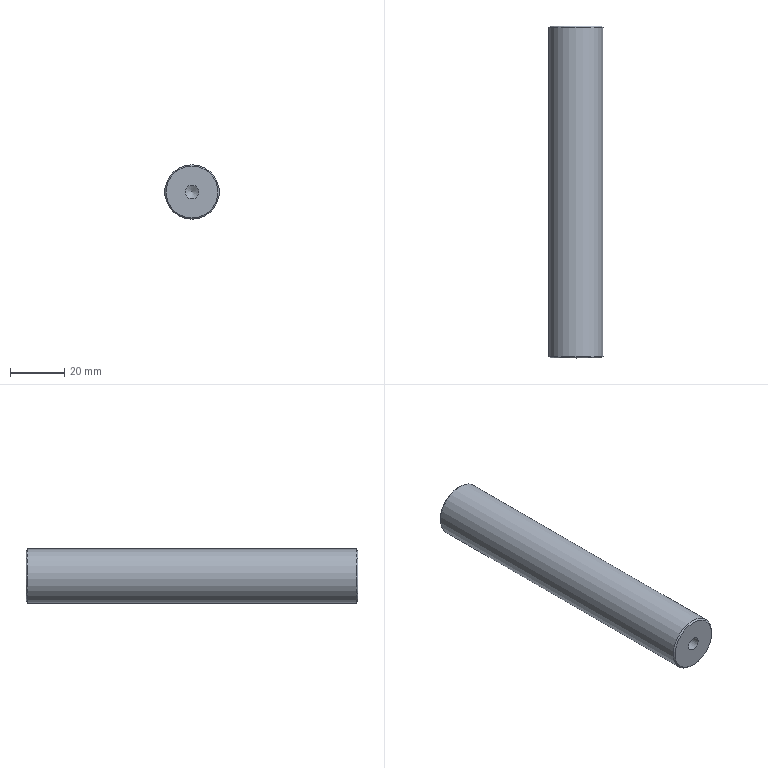Part | NX | 1 solid | 9 faces | box 20 x 122 x 20 mm | volume 37625 mm3 | cone 4 | cylinder 3 | plane 2 | commonest cylinder face diameters 5 x2 20 x1
STEP:
#1=CARTESIAN_POINT('',(0.,60.5,10.));
#2=VERTEX_POINT('',#1);
#3=CARTESIAN_POINT('',(0.,60.5,0.));
#4=DIRECTION('',(0.,1.,0.));
#5=DIRECTION('',(0.,0.,1.));
#6=AXIS2_PLACEMENT_3D('',#3,#4,#5);
#7=CIRCLE('',#6,10.);
#8=EDGE_CURVE('',#2,#2,#7,.F.);
#9=ORIENTED_EDGE('',*,*,#8,.T.);
#10=EDGE_LOOP('',(#9));
#11=FACE_BOUND('',#10,.T.);
#12=CARTESIAN_POINT('',(0.,-60.5,10.));
#13=VERTEX_POINT('',#12);
#14=CARTESIAN_POINT('',(0.,-60.5,0.));
#15=DIRECTION('',(0.,1.,0.));
#16=DIRECTION('',(0.,0.,1.));
#17=AXIS2_PLACEMENT_3D('',#14,#15,#16);
#18=CIRCLE('',#17,10.);
#19=EDGE_CURVE('',#13,#13,#18,.T.);
#20=ORIENTED_EDGE('',*,*,#19,.T.);
#21=EDGE_LOOP('',(#20));
#22=FACE_BOUND('',#21,.T.);
#23=CARTESIAN_POINT('',(0.,61.,0.));
#24=DIRECTION('',(0.,-1.,0.));
#25=DIRECTION('',(0.,0.,-1.));
#26=AXIS2_PLACEMENT_3D('',#23,#24,#25);
#27=CYLINDRICAL_SURFACE('',#26,10.);
#28=ADVANCED_FACE('',(#11,#22),#27,.T.);
#29=CARTESIAN_POINT('',(0.,61.,9.5));
#30=VERTEX_POINT('',#29);
#31=CARTESIAN_POINT('',(0.,61.,0.));
#32=DIRECTION('',(0.,1.,0.));
#33=DIRECTION('',(0.,0.,1.));
#34=AXIS2_PLACEMENT_3D('',#31,#32,#33);
#35=CIRCLE('',#34,9.5);
#36=EDGE_CURVE('',#30,#30,#35,.T.);
#37=ORIENTED_EDGE('',*,*,#36,.T.);
#38=EDGE_LOOP('',(#37));
#39=FACE_BOUND('',#38,.T.);
#40=CARTESIAN_POINT('',(0.,61.,2.5));
#41=VERTEX_POINT('',#40);
#42=CARTESIAN_POINT('',(0.,61.,0.));
#43=DIRECTION('',(0.,1.,0.));
#44=DIRECTION('',(0.,0.,1.));
#45=AXIS2_PLACEMENT_3D('',#42,#43,#44);
#46=CIRCLE('',#45,2.5);
#47=EDGE_CURVE('',#41,#41,#46,.T.);
#48=ORIENTED_EDGE('',*,*,#47,.F.);
#49=EDGE_LOOP('',(#48));
#50=FACE_BOUND('',#49,.T.);
#51=CARTESIAN_POINT('',(0.,61.,0.));
#52=DIRECTION('',(0.,1.,0.));
#53=DIRECTION('',(0.,0.,1.));
#54=AXIS2_PLACEMENT_3D('',#51,#52,#53);
#55=PLANE('',#54);
#56=ADVANCED_FACE('',(#39,#50),#55,.T.);
#57=CARTESIAN_POINT('',(0.,-61.,9.5));
#58=VERTEX_POINT('',#57);
#59=CARTESIAN_POINT('',(0.,-61.,0.));
#60=DIRECTION('',(0.,1.,0.));
#61=DIRECTION('',(0.,0.,1.));
#62=AXIS2_PLACEMENT_3D('',#59,#60,#61);
#63=CIRCLE('',#62,9.5);
#64=EDGE_CURVE('',#58,#58,#63,.F.);
#65=ORIENTED_EDGE('',*,*,#64,.T.);
#66=EDGE_LOOP('',(#65));
#67=FACE_BOUND('',#66,.T.);
#68=CARTESIAN_POINT('',(0.,-61.,-2.5));
#69=VERTEX_POINT('',#68);
#70=CARTESIAN_POINT('',(0.,-61.,0.));
#71=DIRECTION('',(0.,-1.,0.));
#72=DIRECTION('',(0.,0.,-1.));
#73=AXIS2_PLACEMENT_3D('',#70,#71,#72);
#74=CIRCLE('',#73,2.5);
#75=EDGE_CURVE('',#69,#69,#74,.T.);
#76=ORIENTED_EDGE('',*,*,#75,.F.);
#77=EDGE_LOOP('',(#76));
#78=FACE_BOUND('',#77,.T.);
#79=CARTESIAN_POINT('',(0.,-61.,0.));
#80=DIRECTION('',(0.,1.,0.));
#81=DIRECTION('',(0.,0.,1.));
#82=AXIS2_PLACEMENT_3D('',#79,#80,#81);
#83=PLANE('',#82);
#84=ADVANCED_FACE('',(#67,#78),#83,.F.);
#85=CARTESIAN_POINT('',(0.,-42.498,0.));
#86=VERTEX_POINT('',#85);
#87=VERTEX_LOOP('',#86);
#88=FACE_BOUND('',#87,.T.);
#89=CARTESIAN_POINT('',(0.,-44.,-2.5));
#90=VERTEX_POINT('',#89);
#91=CARTESIAN_POINT('',(0.,-44.,0.));
#92=DIRECTION('',(0.,-1.,0.));
#93=DIRECTION('',(0.,0.,-1.));
#94=AXIS2_PLACEMENT_3D('',#91,#92,#93);
#95=CIRCLE('',#94,2.5);
#96=EDGE_CURVE('',#90,#90,#95,.T.);
#97=ORIENTED_EDGE('',*,*,#96,.T.);
#98=EDGE_LOOP('',(#97));
#99=FACE_BOUND('',#98,.T.);
#100=CARTESIAN_POINT('',(0.,-44.,0.));
#101=DIRECTION('',(0.,-1.,0.));
#102=DIRECTION('',(0.,0.,-1.));
#103=AXIS2_PLACEMENT_3D('',#100,#101,#102);
#104=CONICAL_SURFACE('',#103,2.5,1.03);
#105=ADVANCED_FACE('',(#88,#99),#104,.F.);
#106=ORIENTED_EDGE('',*,*,#96,.F.);
#107=EDGE_LOOP('',(#106));
#108=FACE_BOUND('',#107,.T.);
#109=ORIENTED_EDGE('',*,*,#75,.T.);
#110=EDGE_LOOP('',(#109));
#111=FACE_BOUND('',#110,.T.);
#112=CARTESIAN_POINT('',(0.,-61.,0.));
#113=DIRECTION('',(0.,-1.,0.));
#114=DIRECTION('',(0.,0.,-1.));
#115=AXIS2_PLACEMENT_3D('',#112,#113,#114);
#116=CYLINDRICAL_SURFACE('',#115,2.5);
#117=ADVANCED_FACE('',(#108,#111),#116,.F.);
#118=CARTESIAN_POINT('',(0.,42.498,0.));
#119=VERTEX_POINT('',#118);
#120=VERTEX_LOOP('',#119);
#121=FACE_BOUND('',#120,.T.);
#122=CARTESIAN_POINT('',(0.,44.,2.5));
#123=VERTEX_POINT('',#122);
#124=CARTESIAN_POINT('',(0.,44.,0.));
#125=DIRECTION('',(0.,1.,0.));
#126=DIRECTION('',(0.,0.,1.));
#127=AXIS2_PLACEMENT_3D('',#124,#125,#126);
#128=CIRCLE('',#127,2.5);
#129=EDGE_CURVE('',#123,#123,#128,.T.);
#130=ORIENTED_EDGE('',*,*,#129,.T.);
#131=EDGE_LOOP('',(#130));
#132=FACE_BOUND('',#131,.T.);
#133=CARTESIAN_POINT('',(0.,44.,0.));
#134=DIRECTION('',(0.,1.,0.));
#135=DIRECTION('',(0.,0.,1.));
#136=AXIS2_PLACEMENT_3D('',#133,#134,#135);
#137=CONICAL_SURFACE('',#136,2.5,1.03);
#138=ADVANCED_FACE('',(#121,#132),#137,.F.);
#139=ORIENTED_EDGE('',*,*,#129,.F.);
#140=EDGE_LOOP('',(#139));
#141=FACE_BOUND('',#140,.T.);
#142=ORIENTED_EDGE('',*,*,#47,.T.);
#143=EDGE_LOOP('',(#142));
#144=FACE_BOUND('',#143,.T.);
#145=CARTESIAN_POINT('',(0.,61.,0.));
#146=DIRECTION('',(0.,1.,0.));
#147=DIRECTION('',(0.,0.,1.));
#148=AXIS2_PLACEMENT_3D('',#145,#146,#147);
#149=CYLINDRICAL_SURFACE('',#148,2.5);
#150=ADVANCED_FACE('',(#141,#144),#149,.F.);
#151=ORIENTED_EDGE('',*,*,#8,.F.);
#152=EDGE_LOOP('',(#151));
#153=FACE_BOUND('',#152,.T.);
#154=ORIENTED_EDGE('',*,*,#36,.F.);
#155=EDGE_LOOP('',(#154));
#156=FACE_BOUND('',#155,.T.);
#157=CARTESIAN_POINT('',(0.,61.,0.));
#158=DIRECTION('',(0.,-1.,0.));
#159=DIRECTION('',(0.,0.,-1.));
#160=AXIS2_PLACEMENT_3D('',#157,#158,#159);
#161=CONICAL_SURFACE('',#160,9.5,0.7854);
#162=ADVANCED_FACE('',(#153,#156),#161,.T.);
#163=ORIENTED_EDGE('',*,*,#64,.F.);
#164=EDGE_LOOP('',(#163));
#165=FACE_BOUND('',#164,.T.);
#166=ORIENTED_EDGE('',*,*,#19,.F.);
#167=EDGE_LOOP('',(#166));
#168=FACE_BOUND('',#167,.T.);
#169=CARTESIAN_POINT('',(0.,-60.5,0.));
#170=DIRECTION('',(0.,1.,0.));
#171=DIRECTION('',(0.,0.,1.));
#172=AXIS2_PLACEMENT_3D('',#169,#170,#171);
#173=CONICAL_SURFACE('',#172,10.,0.7854);
#174=ADVANCED_FACE('',(#165,#168),#173,.T.);
#175=CLOSED_SHELL('',(#28,#56,#84,#105,#117,#138,#150,#162,#174));
#176=MANIFOLD_SOLID_BREP('',#175);
#177=(LENGTH_UNIT()NAMED_UNIT(*)SI_UNIT(.MILLI.,.METRE.));
#178=UNCERTAINTY_MEASURE_WITH_UNIT(LENGTH_MEASURE(0.00001),#177,'','');
#179=(NAMED_UNIT(*)PLANE_ANGLE_UNIT()SI_UNIT($,.RADIAN.));
#180=(NAMED_UNIT(*)SI_UNIT($,.STERADIAN.)SOLID_ANGLE_UNIT());
#181=(GEOMETRIC_REPRESENTATION_CONTEXT(3)GLOBAL_UNCERTAINTY_ASSIGNED_CONTEXT((#178))GLOBAL_UNIT_ASSIGNED_CONTEXT((#177,#179,#180))REPRESENTATION_CONTEXT('',''));
#182=ADVANCED_BREP_SHAPE_REPRESENTATION('',(#176),#181);